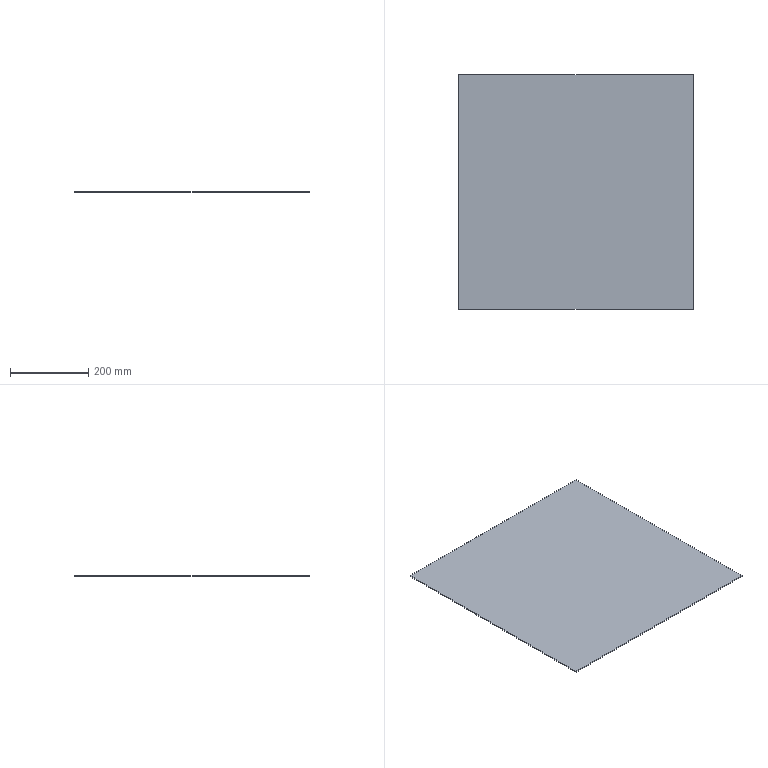Part | SolidWorks | features Extrusion 1 | 1 solid | 6 faces | box 600 x 600 x 2 mm | volume 720000 mm3 | plane 6
STEP:
#1=CARTESIAN_POINT('',(300.,-300.,0.));
#2=VERTEX_POINT('',#1);
#3=CARTESIAN_POINT('',(300.,300.,0.));
#4=VERTEX_POINT('',#3);
#5=CARTESIAN_POINT('',(300.,300.,0.));
#6=DIRECTION('',(0.,1.,0.));
#7=VECTOR('',#6,1000.);
#8=LINE('',#5,#7);
#9=EDGE_CURVE('',#2,#4,#8,.T.);
#10=ORIENTED_EDGE('',*,*,#9,.T.);
#11=CARTESIAN_POINT('',(300.,300.,2.));
#12=VERTEX_POINT('',#11);
#13=CARTESIAN_POINT('',(300.,300.,2.));
#14=DIRECTION('',(0.,0.,-1.));
#15=VECTOR('',#14,1000.);
#16=LINE('',#13,#15);
#17=EDGE_CURVE('',#12,#4,#16,.T.);
#18=ORIENTED_EDGE('',*,*,#17,.F.);
#19=CARTESIAN_POINT('',(300.,-300.,2.));
#20=VERTEX_POINT('',#19);
#21=CARTESIAN_POINT('',(300.,300.,2.));
#22=DIRECTION('',(0.,1.,0.));
#23=VECTOR('',#22,1000.);
#24=LINE('',#21,#23);
#25=EDGE_CURVE('',#20,#12,#24,.T.);
#26=ORIENTED_EDGE('',*,*,#25,.F.);
#27=CARTESIAN_POINT('',(300.,-300.,2.));
#28=DIRECTION('',(0.,0.,-1.));
#29=VECTOR('',#28,1000.);
#30=LINE('',#27,#29);
#31=EDGE_CURVE('',#20,#2,#30,.T.);
#32=ORIENTED_EDGE('',*,*,#31,.T.);
#33=EDGE_LOOP('',(#10,#18,#26,#32));
#34=FACE_OUTER_BOUND('',#33,.T.);
#35=CARTESIAN_POINT('',(300.,300.,2.));
#36=DIRECTION('',(-1.,0.,0.));
#37=DIRECTION('',(0.,-1.,0.));
#38=AXIS2_PLACEMENT_3D('',#35,#36,#37);
#39=PLANE('',#38);
#40=ADVANCED_FACE('',(#34),#39,.F.);
#41=CARTESIAN_POINT('',(-300.,300.,0.));
#42=VERTEX_POINT('',#41);
#43=CARTESIAN_POINT('',(-300.,300.,0.));
#44=DIRECTION('',(-1.,0.,0.));
#45=VECTOR('',#44,1000.);
#46=LINE('',#43,#45);
#47=EDGE_CURVE('',#4,#42,#46,.T.);
#48=ORIENTED_EDGE('',*,*,#47,.T.);
#49=CARTESIAN_POINT('',(-300.,300.,2.));
#50=VERTEX_POINT('',#49);
#51=CARTESIAN_POINT('',(-300.,300.,2.));
#52=DIRECTION('',(0.,0.,-1.));
#53=VECTOR('',#52,1000.);
#54=LINE('',#51,#53);
#55=EDGE_CURVE('',#50,#42,#54,.T.);
#56=ORIENTED_EDGE('',*,*,#55,.F.);
#57=CARTESIAN_POINT('',(-300.,300.,2.));
#58=DIRECTION('',(-1.,0.,0.));
#59=VECTOR('',#58,1000.);
#60=LINE('',#57,#59);
#61=EDGE_CURVE('',#12,#50,#60,.T.);
#62=ORIENTED_EDGE('',*,*,#61,.F.);
#63=ORIENTED_EDGE('',*,*,#17,.T.);
#64=EDGE_LOOP('',(#48,#56,#62,#63));
#65=FACE_OUTER_BOUND('',#64,.T.);
#66=CARTESIAN_POINT('',(-300.,300.,2.));
#67=DIRECTION('',(0.,-1.,0.));
#68=DIRECTION('',(0.,0.,-1.));
#69=AXIS2_PLACEMENT_3D('',#66,#67,#68);
#70=PLANE('',#69);
#71=ADVANCED_FACE('',(#65),#70,.F.);
#72=CARTESIAN_POINT('',(-300.,-300.,0.));
#73=VERTEX_POINT('',#72);
#74=CARTESIAN_POINT('',(-300.,300.,0.));
#75=DIRECTION('',(0.,-1.,0.));
#76=VECTOR('',#75,1000.);
#77=LINE('',#74,#76);
#78=EDGE_CURVE('',#42,#73,#77,.T.);
#79=ORIENTED_EDGE('',*,*,#78,.T.);
#80=CARTESIAN_POINT('',(-300.,-300.,2.));
#81=VERTEX_POINT('',#80);
#82=CARTESIAN_POINT('',(-300.,-300.,2.));
#83=DIRECTION('',(0.,0.,-1.));
#84=VECTOR('',#83,1000.);
#85=LINE('',#82,#84);
#86=EDGE_CURVE('',#81,#73,#85,.T.);
#87=ORIENTED_EDGE('',*,*,#86,.F.);
#88=CARTESIAN_POINT('',(-300.,300.,2.));
#89=DIRECTION('',(0.,-1.,0.));
#90=VECTOR('',#89,1000.);
#91=LINE('',#88,#90);
#92=EDGE_CURVE('',#50,#81,#91,.T.);
#93=ORIENTED_EDGE('',*,*,#92,.F.);
#94=ORIENTED_EDGE('',*,*,#55,.T.);
#95=EDGE_LOOP('',(#79,#87,#93,#94));
#96=FACE_OUTER_BOUND('',#95,.T.);
#97=CARTESIAN_POINT('',(-300.,300.,2.));
#98=DIRECTION('',(1.,0.,0.));
#99=DIRECTION('',(0.,1.,0.));
#100=AXIS2_PLACEMENT_3D('',#97,#98,#99);
#101=PLANE('',#100);
#102=ADVANCED_FACE('',(#96),#101,.F.);
#103=CARTESIAN_POINT('',(-300.,-300.,0.));
#104=DIRECTION('',(1.,0.,0.));
#105=VECTOR('',#104,1000.);
#106=LINE('',#103,#105);
#107=EDGE_CURVE('',#73,#2,#106,.T.);
#108=ORIENTED_EDGE('',*,*,#107,.T.);
#109=ORIENTED_EDGE('',*,*,#31,.F.);
#110=CARTESIAN_POINT('',(-300.,-300.,2.));
#111=DIRECTION('',(1.,0.,0.));
#112=VECTOR('',#111,1000.);
#113=LINE('',#110,#112);
#114=EDGE_CURVE('',#81,#20,#113,.T.);
#115=ORIENTED_EDGE('',*,*,#114,.F.);
#116=ORIENTED_EDGE('',*,*,#86,.T.);
#117=EDGE_LOOP('',(#108,#109,#115,#116));
#118=FACE_OUTER_BOUND('',#117,.T.);
#119=CARTESIAN_POINT('',(-300.,-300.,2.));
#120=DIRECTION('',(0.,1.,0.));
#121=DIRECTION('',(0.,0.,1.));
#122=AXIS2_PLACEMENT_3D('',#119,#120,#121);
#123=PLANE('',#122);
#124=ADVANCED_FACE('',(#118),#123,.F.);
#125=ORIENTED_EDGE('',*,*,#25,.T.);
#126=ORIENTED_EDGE('',*,*,#61,.T.);
#127=ORIENTED_EDGE('',*,*,#92,.T.);
#128=ORIENTED_EDGE('',*,*,#114,.T.);
#129=EDGE_LOOP('',(#125,#126,#127,#128));
#130=FACE_OUTER_BOUND('',#129,.T.);
#131=CARTESIAN_POINT('',(0.,0.,2.));
#132=DIRECTION('',(0.,0.,1.));
#133=DIRECTION('',(1.,0.,0.));
#134=AXIS2_PLACEMENT_3D('',#131,#132,#133);
#135=PLANE('',#134);
#136=ADVANCED_FACE('',(#130),#135,.T.);
#137=ORIENTED_EDGE('',*,*,#9,.F.);
#138=ORIENTED_EDGE('',*,*,#107,.F.);
#139=ORIENTED_EDGE('',*,*,#78,.F.);
#140=ORIENTED_EDGE('',*,*,#47,.F.);
#141=EDGE_LOOP('',(#137,#138,#139,#140));
#142=FACE_OUTER_BOUND('',#141,.T.);
#143=CARTESIAN_POINT('',(0.,0.,0.));
#144=DIRECTION('',(0.,0.,1.));
#145=DIRECTION('',(1.,0.,0.));
#146=AXIS2_PLACEMENT_3D('',#143,#144,#145);
#147=PLANE('',#146);
#148=ADVANCED_FACE('',(#142),#147,.F.);
#149=CLOSED_SHELL('',(#40,#71,#102,#124,#136,#148));
#150=MANIFOLD_SOLID_BREP('',#149);
#151=CARTESIAN_POINT('',(0.,0.,0.));
#152=DIRECTION('',(0.,0.,1.));
#153=DIRECTION('',(1.,0.,0.));
#154=AXIS2_PLACEMENT_3D('',#151,#152,#153);
#155=(LENGTH_UNIT()NAMED_UNIT(*)SI_UNIT(.MILLI.,.METRE.));
#156=UNCERTAINTY_MEASURE_WITH_UNIT(LENGTH_MEASURE(0.00001),#155,'','');
#157=(NAMED_UNIT(*)PLANE_ANGLE_UNIT()SI_UNIT($,.RADIAN.));
#158=(NAMED_UNIT(*)SI_UNIT($,.STERADIAN.)SOLID_ANGLE_UNIT());
#159=(GEOMETRIC_REPRESENTATION_CONTEXT(3)GLOBAL_UNCERTAINTY_ASSIGNED_CONTEXT((#156))GLOBAL_UNIT_ASSIGNED_CONTEXT((#155,#157,#158))REPRESENTATION_CONTEXT('',''));
#160=ADVANCED_BREP_SHAPE_REPRESENTATION('',(#150,#154),#159);